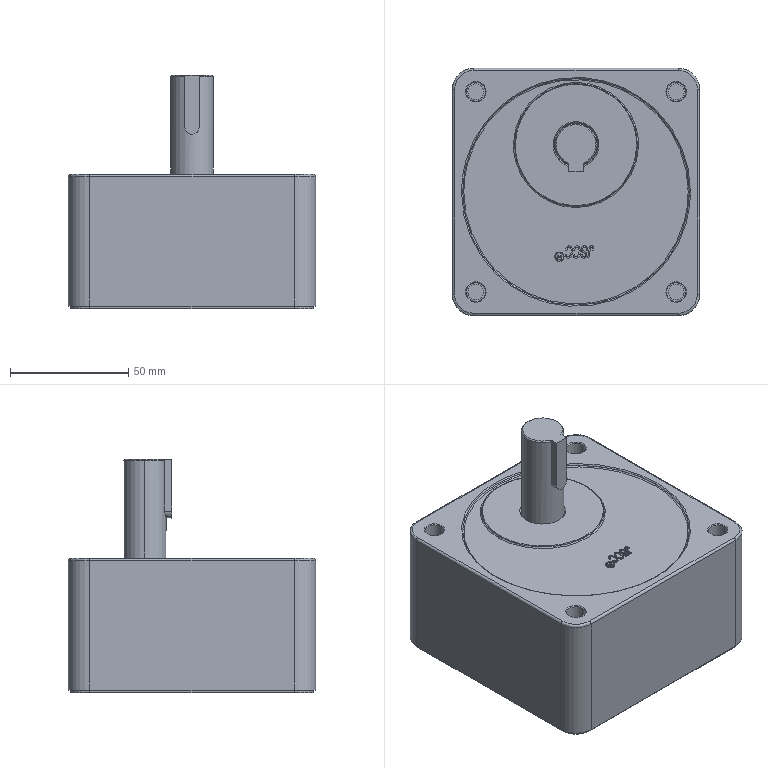Part | SolidWorks | features BaseBody 2 | 2 solids | 246 faces | box 104.8 x 104.8 x 99 mm | volume 576942 mm3 | spline 86 | plane 85 | cylinder 62 | cone 13 | commonest cylinder face diameters 6.7 x16 8 x16 18 x6 0.5 x4 2 x4 16 x4